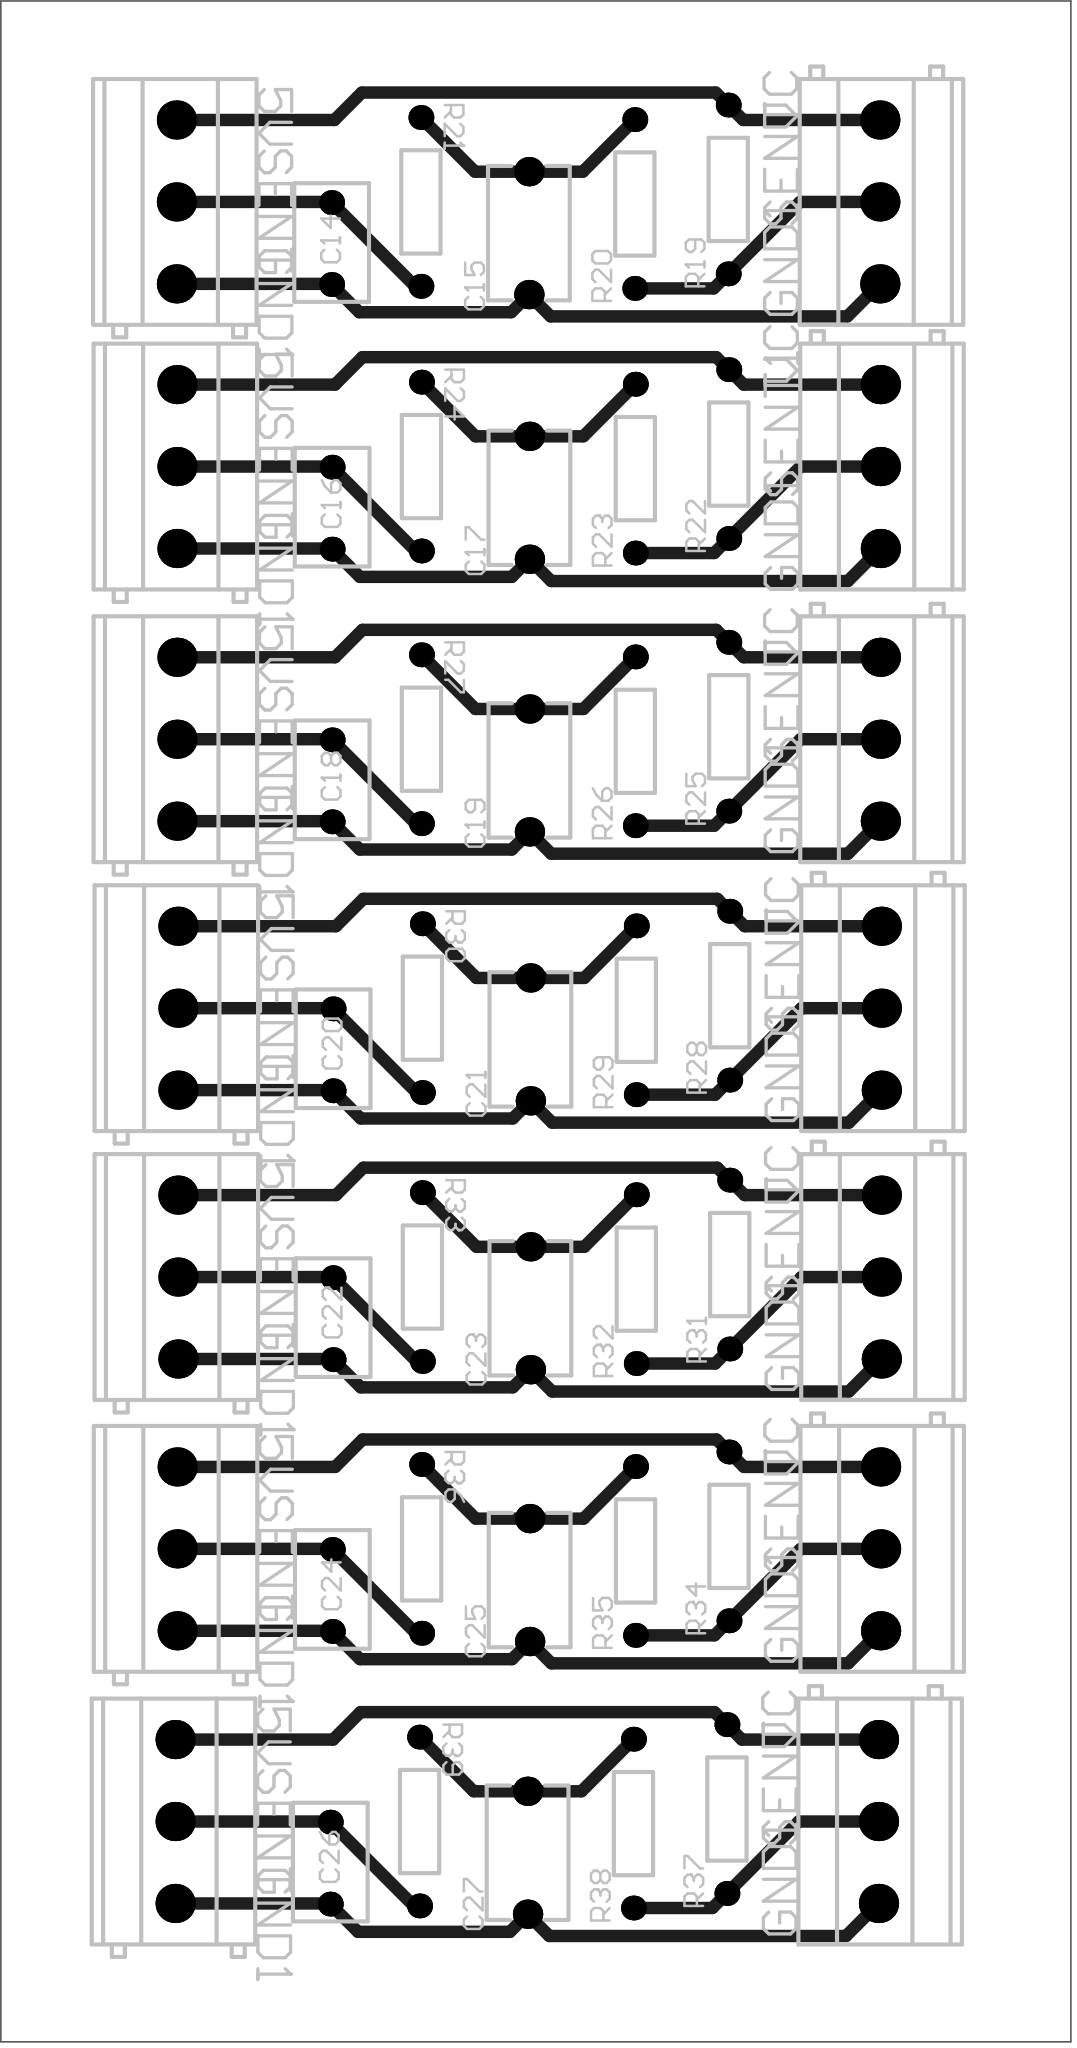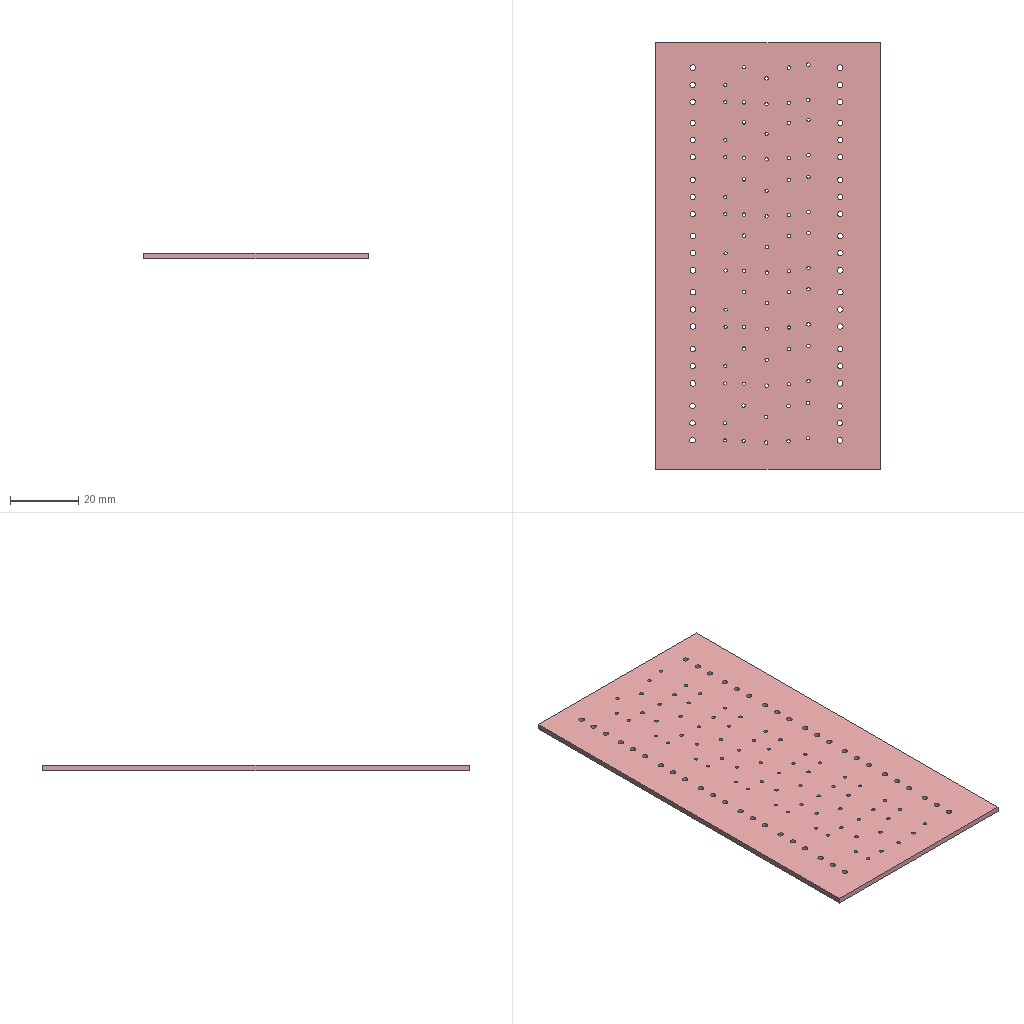Circuit board layout | Altium Designer | box 65.4 x 124.5 x 1.6 mm
Layer stack:
# Altium Designer layer stack of  (unit mm; dielectric type: 0 none, 1 core, 2 prepreg, 3 surface material)
index,name,kind,layer,copper_thickness_mm,dielectric_type,dielectric_thickness_mm,dielectric_material,dielectric_constant
0,Top Paste Mask Layer,other,,,,,,
1,Top Silkscreen Layer,other,,,,,,
2,Top Solder Mask Layer,dielectric,,,3,0.01,,3.3
3,Top Layer,copper,Top Layer,0.035,,,,
4,Dielectric1,dielectric,,,3,1.51,FR4,4.5
5,Bottom Layer,copper,Bottom Layer,0.035,,,,
6,Bottom Solder Mask Layer,dielectric,,,3,0.01,,3.3
7,Bottom Silkscreen Layer,other,,,,,,
8,Bottom Paste Mask Layer,other,,,,,,
# drill layer pairs: low layer,high layer
drill_pair,Top Layer,Bottom Layer
Part placement:
Designator,Comment,Layer,Footprint,Center-X(mm),Center-Y(mm),Rotation
C14,220pF,TopLayer,CAP-TH_L7.2-W4.5-P5.00-D0.5,96.43,185.928,90
C15,2.2nF,TopLayer,CAP-TH_L8.0-W5.0-P7.50-D1.0,108.495,186.563,90
C16,220pF,TopLayer,CAP-TH_L7.2-W4.5-P5.00-D0.5,96.463,169.78,90
C17,2.2nF,TopLayer,CAP-TH_L8.0-W5.0-P7.50-D1.0,108.528,170.415,90
C18,220pF,TopLayer,CAP-TH_L7.2-W4.5-P5.00-D0.5,96.463,153.143,90
C19,2.2nF,TopLayer,CAP-TH_L8.0-W5.0-P7.50-D1.0,108.528,153.778,90
C20,220pF,TopLayer,CAP-TH_L7.2-W4.5-P5.00-D0.5,96.522,136.732,90
C21,2.2nF,TopLayer,CAP-TH_L8.0-W5.0-P7.50-D1.0,108.587,137.367,90
C22,220pF,TopLayer,CAP-TH_L7.2-W4.5-P5.00-D0.5,96.522,120.326,90
C23,2.2nF,TopLayer,CAP-TH_L8.0-W5.0-P7.50-D1.0,108.587,120.961,90
C24,220pF,TopLayer,CAP-TH_L7.2-W4.5-P5.00-D0.5,96.476,103.74,90
C25,2.2nF,TopLayer,CAP-TH_L8.0-W5.0-P7.50-D1.0,108.541,104.375,90
C26,220pF,TopLayer,CAP-TH_L7.2-W4.5-P5.00-D0.5,96.349,87.103,90
C27,2.2nF,TopLayer,CAP-TH_L8.0-W5.0-P7.50-D1.0,108.414,87.738,90
R19,51kΩ,TopLayer,Res_1/4W,120.687,189.23,90
R20,390Ω,TopLayer,Res_1/4W,114.972,188.341,90
R21,3.6kΩ,TopLayer,Res_1/4W,101.891,188.468,270
R22,51kΩ,TopLayer,Res_1/4W,120.72,173.082,90
R23,390Ω,TopLayer,Res_1/4W,115.005,172.193,90
R24,3.6kΩ,TopLayer,Res_1/4W,101.924,172.32,270
R25,51kΩ,TopLayer,Res_1/4W,120.72,156.445,90
R26,390Ω,TopLayer,Res_1/4W,115.005,155.556,90
R27,3.6kΩ,TopLayer,Res_1/4W,101.924,155.683,270
R28,51kΩ,TopLayer,Res_1/4W,120.779,140.034,90
R29,390Ω,TopLayer,Res_1/4W,115.064,139.145,90
R30,3.6kΩ,TopLayer,Res_1/4W,101.983,139.272,270
R31,51kΩ,TopLayer,Res_1/4W,120.779,123.628,90
R32,390Ω,TopLayer,Res_1/4W,115.064,122.739,90
R33,3.6kΩ,TopLayer,Res_1/4W,101.983,122.866,270
R34,51kΩ,TopLayer,Res_1/4W,120.733,107.042,90
R35,390Ω,TopLayer,Res_1/4W,115.018,106.153,90
R36,3.6kΩ,TopLayer,Res_1/4W,101.937,106.28,270
R37,51kΩ,TopLayer,Res_1/4W,120.606,90.405,90
R38,390Ω,TopLayer,Res_1/4W,114.891,89.516,90
R39,3.6kΩ,TopLayer,Res_1/4W,101.81,89.643,270
U14,KF128L-5.0-3P,TopLayer,CONN-TH_3P-P5.00_KF128L-5.0-3P,129.958,188.468,90
U15,KF128L-5.0-3P,TopLayer,CONN-TH_3P-P5.00_KF128L-5.0-3P,86.941,188.468,270
U17,KF128L-5.0-3P,TopLayer,CONN-TH_3P-P5.00_KF128L-5.0-3P,86.974,172.321,270
U18,KF128L-5.0-3P,TopLayer,CONN-TH_3P-P5.00_KF128L-5.0-3P,129.991,155.683,90
U19,KF128L-5.0-3P,TopLayer,CONN-TH_3P-P5.00_KF128L-5.0-3P,86.974,155.684,270
U20,KF128L-5.0-3P,TopLayer,CONN-TH_3P-P5.00_KF128L-5.0-3P,130.05,139.272,90
U21,KF128L-5.0-3P,TopLayer,CONN-TH_3P-P5.00_KF128L-5.0-3P,87.032,139.272,270
U22,KF128L-5.0-3P,TopLayer,CONN-TH_3P-P5.00_KF128L-5.0-3P,130.05,122.866,90
U16,KF128L-5.0-3P,TopLayer,CONN-TH_3P-P5.00_KF128L-5.0-3P,129.991,172.32,90
U23,KF128L-5.0-3P,TopLayer,CONN-TH_3P-P5.00_KF128L-5.0-3P,87.032,122.866,270
U24,KF128L-5.0-3P,TopLayer,CONN-TH_3P-P5.00_KF128L-5.0-3P,130.004,106.28,90
U25,KF128L-5.0-3P,TopLayer,CONN-TH_3P-P5.00_KF128L-5.0-3P,86.987,106.281,270
U26,KF128L-5.0-3P,TopLayer,CONN-TH_3P-P5.00_KF128L-5.0-3P,129.877,89.643,90
U27,KF128L-5.0-3P,TopLayer,CONN-TH_3P-P5.00_KF128L-5.0-3P,86.86,89.644,270
Pad and via stacks:
# Altium Designer via and pad stacks of  (unit mm). Each distinct definition once, with the count of objects using it.
# via: kind,start_layer,end_layer,hole_mm,diameter_mm,mode(0 simple;1 top-mid-bottom;2 full stack),diameter_per_layer,count,example_net
# pad: kind,layer,hole_mm,hole_type(0 round;1 square;2 slot),plating,top_size,top_shape(1 round;2 rect;3 octagon;9 rounded rect),mid_size,bottom_size,mode,footprint,size_per_layer,count,example
pad,Multi-Layer,0.9144,0,plated,1.524x1.524,1,1.524x1.524,1.524x1.524,0,CAP-TH_L7.2-W4.5-P5.00-D0.5,,14,C14.1
pad,Multi-Layer,1,0,plated,1.8x1.8,1,1.8x1.8,1.8x1.8,0,CAP-TH_L8.0-W5.0-P7.50-D1.0,,14,C15.1
pad,Multi-Layer,1,0,plated,1.524x1.524,1,1.524x1.524,1.524x1.524,0,Res_1/4W,,42,R19.1
pad,Multi-Layer,1.6,0,plated,2.4x2.4,1,2.4x2.4,2.4x2.4,0,CONN-TH_3P-P5.00_KF128L-5.0-3P,,42,U14.1
Design rules, without the lines most boards share:
# Altium Designer design rules of  (exported by Altium Designer, unit mm)
# columns: name | kind | enabled | priority | scope1 | scope2 | descriptor | typed fields (field=value)
copperThickness1oz_2 | 2 | enabled | 2 | All | All | Width Constraint (Min=5mil) (Max=100mil) (Preferred=30mil) (All) |
viaSize | 11 | enabled | 1 | All | All | Routing Via (MinHoleWidth=11.811mil) (MaxHoleWidth=248.032mil) (PreferredHoleWidth=12.008mil) (MinWidth=19.685mil) (MaxWidth=393.701mil) (PreferedWidth=24.016mil) (All) | via_min_hole=0.3 via_max_hole=6.3 via_preferred_diameter=0.61 via_preferred_hole=0.305
solderMaskExpansion | 13 | enabled | 2 | All | All | Solder Mask Expansion (Expansion =2.008mil) (All) | expansion=0.051